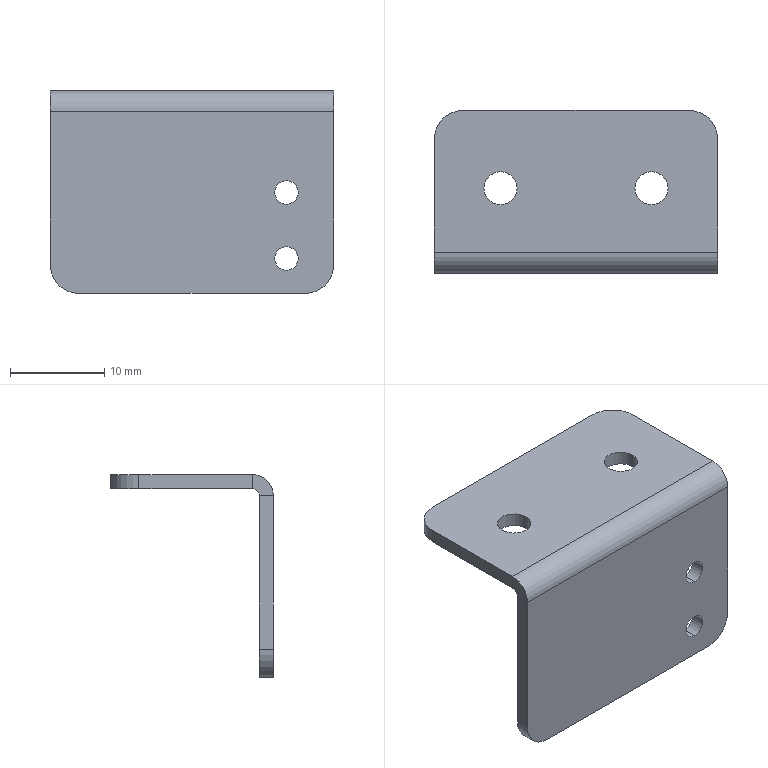Part | STEP file | PN_0030(Default) | 1 solid | 26 faces | box 30 x 17.237 x 21.5 mm | volume 1592 mm3 | cylinder 14 | plane 12 | commonest cylinder face diameters 2.5 x4 3.5 x4 6 x4 1.473 x1 4.473 x1